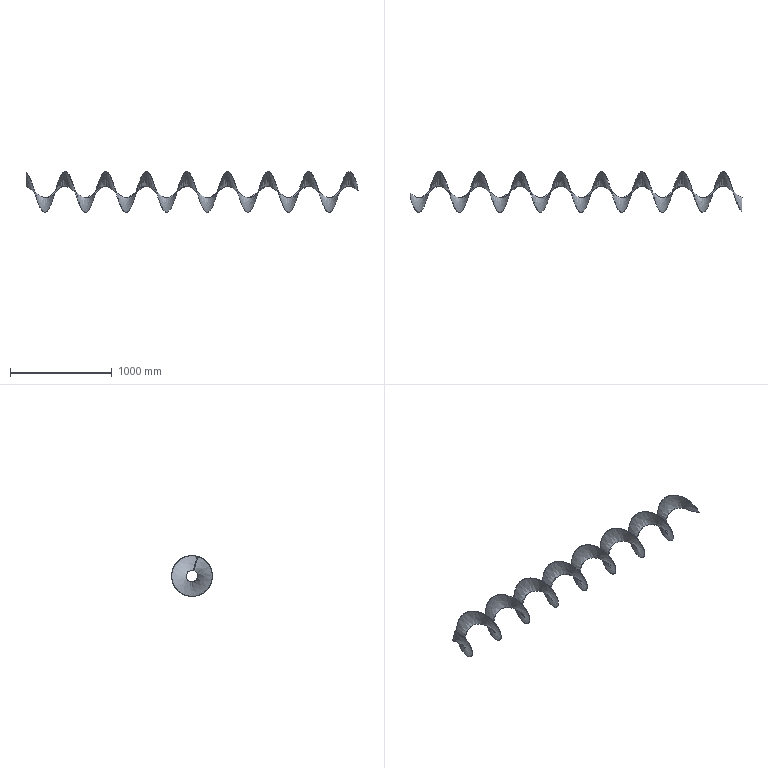Part | STEP file | Input 32 | 1 solid | 4 faces | box 3271 x 400.356 x 400.198 mm | volume 12173770 mm3 | spline 2 | plane 2